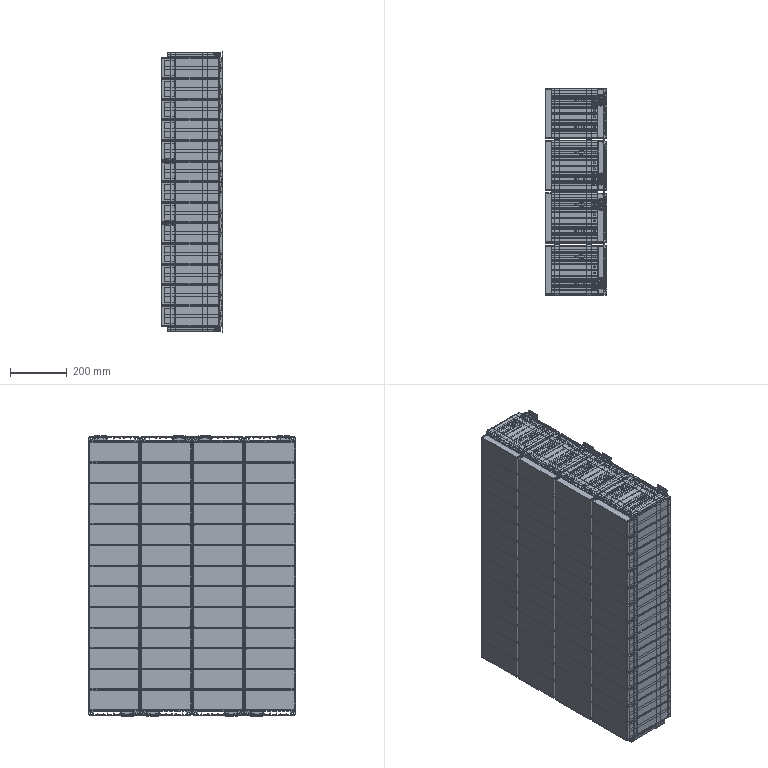Part | NX | features BREP 21 | 305 solids | 51406 faces | volume 139078395 mm3 | plane 31206 | cylinder 18888 | cone 636 | torus 316 | spline 248 | sphere 112 | commonest cylinder face diameters 8 x3992 2 x2432 6 x1764 4 x1628 0.4 x944 3 x832